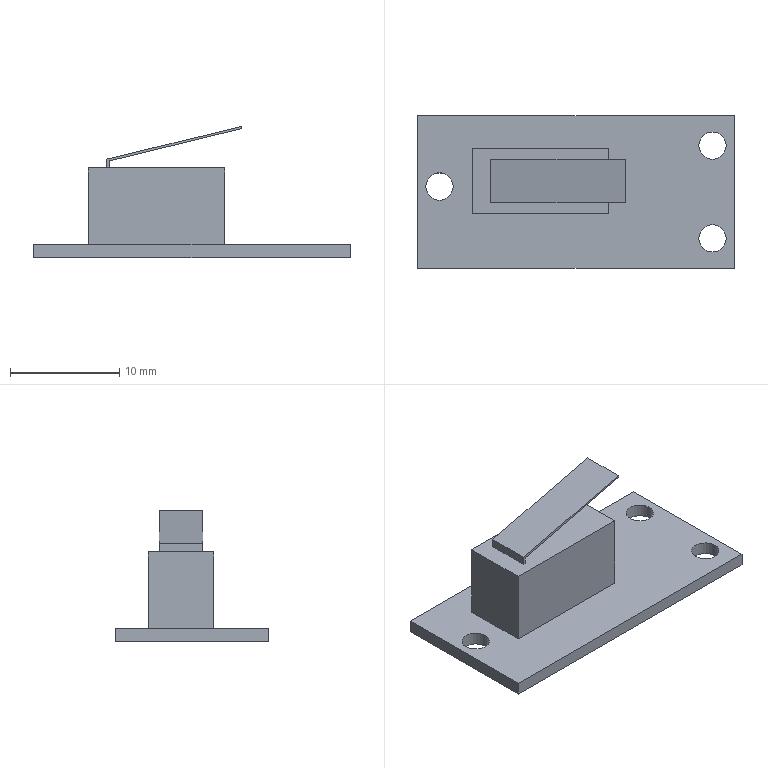Part | STEP file | Q7C1213W | 1 solid | 21 faces | box 29 x 14 x 12 mm | volume 1005 mm3 | plane 18 | cylinder 3 | commonest cylinder face diameters 2.5 x3
STEP:
#1=CARTESIAN_POINT('',(0.,0.,0.));
#2=DIRECTION('',(0.,0.,1.));
#3=DIRECTION('',(1.,0.,0.));
#4=AXIS2_PLACEMENT_3D('',#1,#2,#3);
#5=CARTESIAN_POINT('',(-11.25,0.5,1.2));
#6=VERTEX_POINT('',#5);
#7=CARTESIAN_POINT('',(-12.5,0.5,1.2));
#8=DIRECTION('',(0.,0.,1.));
#9=DIRECTION('',(1.,0.,0.));
#10=AXIS2_PLACEMENT_3D('',#7,#8,#9);
#11=CIRCLE('',#10,1.25);
#12=CARTESIAN_POINT('',(-14.5,-7.,1.2));
#13=DIRECTION('',(0.,0.,1.));
#14=DIRECTION('',(1.,0.,0.));
#15=AXIS2_PLACEMENT_3D('',#12,#13,#14);
#16=PLANE('',#15);
#17=CARTESIAN_POINT('',(2.,7.5));
#18=DIRECTION('',(1.,0.));
#19=AXIS2_PLACEMENT_2D('',#17,#18);
#20=CIRCLE('',#19,1.25);
#21=(GEOMETRIC_REPRESENTATION_CONTEXT(2)PARAMETRIC_REPRESENTATION_CONTEXT()REPRESENTATION_CONTEXT('',''));
#22=DEFINITIONAL_REPRESENTATION('',(#20),#21);
#23=PCURVE('',#16,#22);
#24=CARTESIAN_POINT('',(-12.5,0.5,1.2));
#25=DIRECTION('',(0.,0.,-1.));
#26=DIRECTION('',(-1.,0.,0.));
#27=AXIS2_PLACEMENT_3D('',#24,#25,#26);
#28=CYLINDRICAL_SURFACE('',#27,1.25);
#29=CARTESIAN_POINT('',(9.425,0.));
#30=DIRECTION('',(-1.,0.));
#31=VECTOR('',#30,1.);
#32=LINE('',#29,#31);
#33=(GEOMETRIC_REPRESENTATION_CONTEXT(2)PARAMETRIC_REPRESENTATION_CONTEXT()REPRESENTATION_CONTEXT('',''));
#34=DEFINITIONAL_REPRESENTATION('',(#32),#33);
#35=PCURVE('',#28,#34);
#36=SURFACE_CURVE('',#11,(#23,#35),.PCURVE_S1.);
#37=EDGE_CURVE('',#6,#6,#36,.T.);
#38=ORIENTED_EDGE('',*,*,#37,.F.);
#39=EDGE_LOOP('',(#38));
#40=FACE_BOUND('',#39,.T.);
#41=CARTESIAN_POINT('',(13.75,4.25,1.2));
#42=VERTEX_POINT('',#41);
#43=CARTESIAN_POINT('',(12.5,4.25,1.2));
#44=DIRECTION('',(0.,0.,1.));
#45=DIRECTION('',(1.,0.,0.));
#46=AXIS2_PLACEMENT_3D('',#43,#44,#45);
#47=CIRCLE('',#46,1.25);
#48=CARTESIAN_POINT('',(27.,11.25));
#49=DIRECTION('',(1.,0.));
#50=AXIS2_PLACEMENT_2D('',#48,#49);
#51=CIRCLE('',#50,1.25);
#52=(GEOMETRIC_REPRESENTATION_CONTEXT(2)PARAMETRIC_REPRESENTATION_CONTEXT()REPRESENTATION_CONTEXT('',''));
#53=DEFINITIONAL_REPRESENTATION('',(#51),#52);
#54=PCURVE('',#16,#53);
#55=CARTESIAN_POINT('',(12.5,4.25,1.2));
#56=DIRECTION('',(0.,0.,-1.));
#57=DIRECTION('',(-1.,0.,0.));
#58=AXIS2_PLACEMENT_3D('',#55,#56,#57);
#59=CYLINDRICAL_SURFACE('',#58,1.25);
#60=CARTESIAN_POINT('',(9.425,0.));
#61=DIRECTION('',(-1.,0.));
#62=VECTOR('',#61,1.);
#63=LINE('',#60,#62);
#64=(GEOMETRIC_REPRESENTATION_CONTEXT(2)PARAMETRIC_REPRESENTATION_CONTEXT()REPRESENTATION_CONTEXT('',''));
#65=DEFINITIONAL_REPRESENTATION('',(#63),#64);
#66=PCURVE('',#59,#65);
#67=SURFACE_CURVE('',#47,(#54,#66),.PCURVE_S1.);
#68=EDGE_CURVE('',#42,#42,#67,.T.);
#69=ORIENTED_EDGE('',*,*,#68,.F.);
#70=EDGE_LOOP('',(#69));
#71=FACE_BOUND('',#70,.T.);
#72=CARTESIAN_POINT('',(-14.5,7.,1.2));
#73=VERTEX_POINT('',#72);
#74=CARTESIAN_POINT('',(-14.5,-7.,1.2));
#75=VERTEX_POINT('',#74);
#76=CARTESIAN_POINT('',(-14.5,7.,1.2));
#77=DIRECTION('',(0.,-1.,0.));
#78=VECTOR('',#77,1.);
#79=LINE('',#76,#78);
#80=CARTESIAN_POINT('',(0.,14.));
#81=DIRECTION('',(0.,-1.));
#82=VECTOR('',#81,1.);
#83=LINE('',#80,#82);
#84=(GEOMETRIC_REPRESENTATION_CONTEXT(2)PARAMETRIC_REPRESENTATION_CONTEXT()REPRESENTATION_CONTEXT('',''));
#85=DEFINITIONAL_REPRESENTATION('',(#83),#84);
#86=PCURVE('',#16,#85);
#87=CARTESIAN_POINT('',(-14.5,7.,1.2));
#88=DIRECTION('',(1.,0.,0.));
#89=DIRECTION('',(0.,1.,0.));
#90=AXIS2_PLACEMENT_3D('',#87,#88,#89);
#91=PLANE('',#90);
#92=CARTESIAN_POINT('',(0.,0.));
#93=DIRECTION('',(-1.,0.));
#94=VECTOR('',#93,1.);
#95=LINE('',#92,#94);
#96=(GEOMETRIC_REPRESENTATION_CONTEXT(2)PARAMETRIC_REPRESENTATION_CONTEXT()REPRESENTATION_CONTEXT('',''));
#97=DEFINITIONAL_REPRESENTATION('',(#95),#96);
#98=PCURVE('',#91,#97);
#99=SURFACE_CURVE('',#79,(#86,#98),.PCURVE_S1.);
#100=EDGE_CURVE('',#73,#75,#99,.T.);
#101=ORIENTED_EDGE('',*,*,#100,.T.);
#102=CARTESIAN_POINT('',(14.5,-7.,1.2));
#103=VERTEX_POINT('',#102);
#104=CARTESIAN_POINT('',(-14.5,-7.,1.2));
#105=DIRECTION('',(1.,0.,0.));
#106=VECTOR('',#105,1.);
#107=LINE('',#104,#106);
#108=CARTESIAN_POINT('',(0.,0.));
#109=DIRECTION('',(1.,0.));
#110=VECTOR('',#109,1.);
#111=LINE('',#108,#110);
#112=(GEOMETRIC_REPRESENTATION_CONTEXT(2)PARAMETRIC_REPRESENTATION_CONTEXT()REPRESENTATION_CONTEXT('',''));
#113=DEFINITIONAL_REPRESENTATION('',(#111),#112);
#114=PCURVE('',#16,#113);
#115=CARTESIAN_POINT('',(-14.5,-7.,1.2));
#116=DIRECTION('',(0.,1.,0.));
#117=DIRECTION('',(0.,0.,1.));
#118=AXIS2_PLACEMENT_3D('',#115,#116,#117);
#119=PLANE('',#118);
#120=CARTESIAN_POINT('',(0.,0.));
#121=DIRECTION('',(0.,1.));
#122=VECTOR('',#121,1.);
#123=LINE('',#120,#122);
#124=(GEOMETRIC_REPRESENTATION_CONTEXT(2)PARAMETRIC_REPRESENTATION_CONTEXT()REPRESENTATION_CONTEXT('',''));
#125=DEFINITIONAL_REPRESENTATION('',(#123),#124);
#126=PCURVE('',#119,#125);
#127=SURFACE_CURVE('',#107,(#114,#126),.PCURVE_S1.);
#128=EDGE_CURVE('',#75,#103,#127,.T.);
#129=ORIENTED_EDGE('',*,*,#128,.T.);
#130=CARTESIAN_POINT('',(14.5,7.,1.2));
#131=VERTEX_POINT('',#130);
#132=CARTESIAN_POINT('',(14.5,7.,1.2));
#133=DIRECTION('',(0.,1.,0.));
#134=VECTOR('',#133,1.);
#135=LINE('',#132,#134);
#136=CARTESIAN_POINT('',(29.,14.));
#137=DIRECTION('',(0.,1.));
#138=VECTOR('',#137,1.);
#139=LINE('',#136,#138);
#140=(GEOMETRIC_REPRESENTATION_CONTEXT(2)PARAMETRIC_REPRESENTATION_CONTEXT()REPRESENTATION_CONTEXT('',''));
#141=DEFINITIONAL_REPRESENTATION('',(#139),#140);
#142=PCURVE('',#16,#141);
#143=CARTESIAN_POINT('',(14.5,7.,1.2));
#144=DIRECTION('',(-1.,0.,0.));
#145=DIRECTION('',(0.,-1.,0.));
#146=AXIS2_PLACEMENT_3D('',#143,#144,#145);
#147=PLANE('',#146);
#148=CARTESIAN_POINT('',(0.,0.));
#149=DIRECTION('',(-1.,0.));
#150=VECTOR('',#149,1.);
#151=LINE('',#148,#150);
#152=(GEOMETRIC_REPRESENTATION_CONTEXT(2)PARAMETRIC_REPRESENTATION_CONTEXT()REPRESENTATION_CONTEXT('',''));
#153=DEFINITIONAL_REPRESENTATION('',(#151),#152);
#154=PCURVE('',#147,#153);
#155=SURFACE_CURVE('',#135,(#142,#154),.PCURVE_S1.);
#156=EDGE_CURVE('',#103,#131,#155,.T.);
#157=ORIENTED_EDGE('',*,*,#156,.T.);
#158=CARTESIAN_POINT('',(-14.5,7.,1.2));
#159=DIRECTION('',(-1.,0.,0.));
#160=VECTOR('',#159,1.);
#161=LINE('',#158,#160);
#162=CARTESIAN_POINT('',(0.,14.));
#163=DIRECTION('',(-1.,0.));
#164=VECTOR('',#163,1.);
#165=LINE('',#162,#164);
#166=(GEOMETRIC_REPRESENTATION_CONTEXT(2)PARAMETRIC_REPRESENTATION_CONTEXT()REPRESENTATION_CONTEXT('',''));
#167=DEFINITIONAL_REPRESENTATION('',(#165),#166);
#168=PCURVE('',#16,#167);
#169=CARTESIAN_POINT('',(-14.5,7.,1.2));
#170=DIRECTION('',(0.,-1.,0.));
#171=DIRECTION('',(0.,0.,-1.));
#172=AXIS2_PLACEMENT_3D('',#169,#170,#171);
#173=PLANE('',#172);
#174=CARTESIAN_POINT('',(0.,0.));
#175=DIRECTION('',(0.,-1.));
#176=VECTOR('',#175,1.);
#177=LINE('',#174,#176);
#178=(GEOMETRIC_REPRESENTATION_CONTEXT(2)PARAMETRIC_REPRESENTATION_CONTEXT()REPRESENTATION_CONTEXT('',''));
#179=DEFINITIONAL_REPRESENTATION('',(#177),#178);
#180=PCURVE('',#173,#179);
#181=SURFACE_CURVE('',#161,(#168,#180),.PCURVE_S1.);
#182=EDGE_CURVE('',#131,#73,#181,.T.);
#183=ORIENTED_EDGE('',*,*,#182,.T.);
#184=EDGE_LOOP('',(#101,#129,#157,#183));
#185=FACE_BOUND('',#184,.T.);
#186=CARTESIAN_POINT('',(13.75,-4.25,1.2));
#187=VERTEX_POINT('',#186);
#188=CARTESIAN_POINT('',(12.5,-4.25,1.2));
#189=DIRECTION('',(0.,0.,1.));
#190=DIRECTION('',(1.,0.,0.));
#191=AXIS2_PLACEMENT_3D('',#188,#189,#190);
#192=CIRCLE('',#191,1.25);
#193=CARTESIAN_POINT('',(27.,2.75));
#194=DIRECTION('',(1.,0.));
#195=AXIS2_PLACEMENT_2D('',#193,#194);
#196=CIRCLE('',#195,1.25);
#197=(GEOMETRIC_REPRESENTATION_CONTEXT(2)PARAMETRIC_REPRESENTATION_CONTEXT()REPRESENTATION_CONTEXT('',''));
#198=DEFINITIONAL_REPRESENTATION('',(#196),#197);
#199=PCURVE('',#16,#198);
#200=CARTESIAN_POINT('',(12.5,-4.25,1.2));
#201=DIRECTION('',(0.,0.,-1.));
#202=DIRECTION('',(-1.,0.,0.));
#203=AXIS2_PLACEMENT_3D('',#200,#201,#202);
#204=CYLINDRICAL_SURFACE('',#203,1.25);
#205=CARTESIAN_POINT('',(9.425,0.));
#206=DIRECTION('',(-1.,0.));
#207=VECTOR('',#206,1.);
#208=LINE('',#205,#207);
#209=(GEOMETRIC_REPRESENTATION_CONTEXT(2)PARAMETRIC_REPRESENTATION_CONTEXT()REPRESENTATION_CONTEXT('',''));
#210=DEFINITIONAL_REPRESENTATION('',(#208),#209);
#211=PCURVE('',#204,#210);
#212=SURFACE_CURVE('',#192,(#199,#211),.PCURVE_S1.);
#213=EDGE_CURVE('',#187,#187,#212,.T.);
#214=ORIENTED_EDGE('',*,*,#213,.F.);
#215=EDGE_LOOP('',(#214));
#216=FACE_BOUND('',#215,.T.);
#217=CARTESIAN_POINT('',(-9.5,-2.,1.2));
#218=VERTEX_POINT('',#217);
#219=CARTESIAN_POINT('',(3.,-2.,1.2));
#220=VERTEX_POINT('',#219);
#221=CARTESIAN_POINT('',(-9.5,-2.,1.2));
#222=DIRECTION('',(1.,0.,0.));
#223=VECTOR('',#222,1.);
#224=LINE('',#221,#223);
#225=CARTESIAN_POINT('',(5.,5.));
#226=DIRECTION('',(1.,0.));
#227=VECTOR('',#226,1.);
#228=LINE('',#225,#227);
#229=(GEOMETRIC_REPRESENTATION_CONTEXT(2)PARAMETRIC_REPRESENTATION_CONTEXT()REPRESENTATION_CONTEXT('',''));
#230=DEFINITIONAL_REPRESENTATION('',(#228),#229);
#231=PCURVE('',#16,#230);
#232=CARTESIAN_POINT('',(-9.5,-2.,8.2));
#233=DIRECTION('',(0.,1.,0.));
#234=DIRECTION('',(0.,0.,1.));
#235=AXIS2_PLACEMENT_3D('',#232,#233,#234);
#236=PLANE('',#235);
#237=CARTESIAN_POINT('',(-7.,0.));
#238=DIRECTION('',(0.,1.));
#239=VECTOR('',#238,1.);
#240=LINE('',#237,#239);
#241=(GEOMETRIC_REPRESENTATION_CONTEXT(2)PARAMETRIC_REPRESENTATION_CONTEXT()REPRESENTATION_CONTEXT('',''));
#242=DEFINITIONAL_REPRESENTATION('',(#240),#241);
#243=PCURVE('',#236,#242);
#244=SURFACE_CURVE('',#224,(#231,#243),.PCURVE_S1.);
#245=EDGE_CURVE('',#218,#220,#244,.T.);
#246=ORIENTED_EDGE('',*,*,#245,.F.);
#247=CARTESIAN_POINT('',(-9.5,4.,1.2));
#248=VERTEX_POINT('',#247);
#249=CARTESIAN_POINT('',(-9.5,4.,1.2));
#250=DIRECTION('',(0.,-1.,0.));
#251=VECTOR('',#250,1.);
#252=LINE('',#249,#251);
#253=CARTESIAN_POINT('',(5.,11.));
#254=DIRECTION('',(0.,-1.));
#255=VECTOR('',#254,1.);
#256=LINE('',#253,#255);
#257=(GEOMETRIC_REPRESENTATION_CONTEXT(2)PARAMETRIC_REPRESENTATION_CONTEXT()REPRESENTATION_CONTEXT('',''));
#258=DEFINITIONAL_REPRESENTATION('',(#256),#257);
#259=PCURVE('',#16,#258);
#260=CARTESIAN_POINT('',(-9.5,4.,8.2));
#261=DIRECTION('',(1.,0.,0.));
#262=DIRECTION('',(0.,0.,-1.));
#263=AXIS2_PLACEMENT_3D('',#260,#261,#262);
#264=PLANE('',#263);
#265=CARTESIAN_POINT('',(7.,0.));
#266=DIRECTION('',(0.,-1.));
#267=VECTOR('',#266,1.);
#268=LINE('',#265,#267);
#269=(GEOMETRIC_REPRESENTATION_CONTEXT(2)PARAMETRIC_REPRESENTATION_CONTEXT()REPRESENTATION_CONTEXT('',''));
#270=DEFINITIONAL_REPRESENTATION('',(#268),#269);
#271=PCURVE('',#264,#270);
#272=SURFACE_CURVE('',#252,(#259,#271),.PCURVE_S1.);
#273=EDGE_CURVE('',#248,#218,#272,.T.);
#274=ORIENTED_EDGE('',*,*,#273,.F.);
#275=CARTESIAN_POINT('',(3.,4.,1.2));
#276=VERTEX_POINT('',#275);
#277=CARTESIAN_POINT('',(-9.5,4.,1.2));
#278=DIRECTION('',(-1.,0.,0.));
#279=VECTOR('',#278,1.);
#280=LINE('',#277,#279);
#281=CARTESIAN_POINT('',(5.,11.));
#282=DIRECTION('',(-1.,0.));
#283=VECTOR('',#282,1.);
#284=LINE('',#281,#283);
#285=(GEOMETRIC_REPRESENTATION_CONTEXT(2)PARAMETRIC_REPRESENTATION_CONTEXT()REPRESENTATION_CONTEXT('',''));
#286=DEFINITIONAL_REPRESENTATION('',(#284),#285);
#287=PCURVE('',#16,#286);
#288=CARTESIAN_POINT('',(-9.5,4.,8.2));
#289=DIRECTION('',(0.,-1.,0.));
#290=DIRECTION('',(0.,0.,-1.));
#291=AXIS2_PLACEMENT_3D('',#288,#289,#290);
#292=PLANE('',#291);
#293=CARTESIAN_POINT('',(7.,0.));
#294=DIRECTION('',(0.,-1.));
#295=VECTOR('',#294,1.);
#296=LINE('',#293,#295);
#297=(GEOMETRIC_REPRESENTATION_CONTEXT(2)PARAMETRIC_REPRESENTATION_CONTEXT()REPRESENTATION_CONTEXT('',''));
#298=DEFINITIONAL_REPRESENTATION('',(#296),#297);
#299=PCURVE('',#292,#298);
#300=SURFACE_CURVE('',#280,(#287,#299),.PCURVE_S1.);
#301=EDGE_CURVE('',#276,#248,#300,.T.);
#302=ORIENTED_EDGE('',*,*,#301,.F.);
#303=CARTESIAN_POINT('',(3.,4.,1.2));
#304=DIRECTION('',(0.,1.,0.));
#305=VECTOR('',#304,1.);
#306=LINE('',#303,#305);
#307=CARTESIAN_POINT('',(17.5,11.));
#308=DIRECTION('',(0.,1.));
#309=VECTOR('',#308,1.);
#310=LINE('',#307,#309);
#311=(GEOMETRIC_REPRESENTATION_CONTEXT(2)PARAMETRIC_REPRESENTATION_CONTEXT()REPRESENTATION_CONTEXT('',''));
#312=DEFINITIONAL_REPRESENTATION('',(#310),#311);
#313=PCURVE('',#16,#312);
#314=CARTESIAN_POINT('',(3.,4.,8.2));
#315=DIRECTION('',(-1.,0.,0.));
#316=DIRECTION('',(0.,0.,1.));
#317=AXIS2_PLACEMENT_3D('',#314,#315,#316);
#318=PLANE('',#317);
#319=CARTESIAN_POINT('',(-7.,0.));
#320=DIRECTION('',(0.,1.));
#321=VECTOR('',#320,1.);
#322=LINE('',#319,#321);
#323=(GEOMETRIC_REPRESENTATION_CONTEXT(2)PARAMETRIC_REPRESENTATION_CONTEXT()REPRESENTATION_CONTEXT('',''));
#324=DEFINITIONAL_REPRESENTATION('',(#322),#323);
#325=PCURVE('',#318,#324);
#326=SURFACE_CURVE('',#306,(#313,#325),.PCURVE_S1.);
#327=EDGE_CURVE('',#220,#276,#326,.T.);
#328=ORIENTED_EDGE('',*,*,#327,.F.);
#329=EDGE_LOOP('',(#246,#274,#302,#328));
#330=FACE_BOUND('',#329,.T.);
#331=ADVANCED_FACE('',(#40,#71,#185,#216,#330),#16,.T.);
#332=CARTESIAN_POINT('',(13.75,-4.25,0.));
#333=VERTEX_POINT('',#332);
#334=CARTESIAN_POINT('',(12.5,-4.25,0.));
#335=DIRECTION('',(0.,0.,1.));
#336=DIRECTION('',(1.,0.,0.));
#337=AXIS2_PLACEMENT_3D('',#334,#335,#336);
#338=CIRCLE('',#337,1.25);
#339=CARTESIAN_POINT('',(-14.5,-7.,0.));
#340=DIRECTION('',(0.,0.,1.));
#341=DIRECTION('',(1.,0.,0.));
#342=AXIS2_PLACEMENT_3D('',#339,#340,#341);
#343=PLANE('',#342);
#344=CARTESIAN_POINT('',(27.,2.75));
#345=DIRECTION('',(1.,0.));
#346=AXIS2_PLACEMENT_2D('',#344,#345);
#347=CIRCLE('',#346,1.25);
#348=(GEOMETRIC_REPRESENTATION_CONTEXT(2)PARAMETRIC_REPRESENTATION_CONTEXT()REPRESENTATION_CONTEXT('',''));
#349=DEFINITIONAL_REPRESENTATION('',(#347),#348);
#350=PCURVE('',#343,#349);
#351=CARTESIAN_POINT('',(9.425,1.2));
#352=DIRECTION('',(-1.,0.));
#353=VECTOR('',#352,1.);
#354=LINE('',#351,#353);
#355=(GEOMETRIC_REPRESENTATION_CONTEXT(2)PARAMETRIC_REPRESENTATION_CONTEXT()REPRESENTATION_CONTEXT('',''));
#356=DEFINITIONAL_REPRESENTATION('',(#354),#355);
#357=PCURVE('',#204,#356);
#358=SURFACE_CURVE('',#338,(#350,#357),.PCURVE_S1.);
#359=EDGE_CURVE('',#333,#333,#358,.T.);
#360=ORIENTED_EDGE('',*,*,#359,.T.);
#361=EDGE_LOOP('',(#360));
#362=FACE_BOUND('',#361,.T.);
#363=CARTESIAN_POINT('',(-14.5,7.,0.));
#364=VERTEX_POINT('',#363);
#365=CARTESIAN_POINT('',(-14.5,-7.,0.));
#366=VERTEX_POINT('',#365);
#367=CARTESIAN_POINT('',(-14.5,7.,0.));
#368=DIRECTION('',(0.,-1.,0.));
#369=VECTOR('',#368,1.);
#370=LINE('',#367,#369);
#371=CARTESIAN_POINT('',(0.,14.));
#372=DIRECTION('',(0.,-1.));
#373=VECTOR('',#372,1.);
#374=LINE('',#371,#373);
#375=(GEOMETRIC_REPRESENTATION_CONTEXT(2)PARAMETRIC_REPRESENTATION_CONTEXT()REPRESENTATION_CONTEXT('',''));
#376=DEFINITIONAL_REPRESENTATION('',(#374),#375);
#377=PCURVE('',#343,#376);
#378=CARTESIAN_POINT('',(0.,-1.2));
#379=DIRECTION('',(-1.,0.));
#380=VECTOR('',#379,1.);
#381=LINE('',#378,#380);
#382=(GEOMETRIC_REPRESENTATION_CONTEXT(2)PARAMETRIC_REPRESENTATION_CONTEXT()REPRESENTATION_CONTEXT('',''));
#383=DEFINITIONAL_REPRESENTATION('',(#381),#382);
#384=PCURVE('',#91,#383);
#385=SURFACE_CURVE('',#370,(#377,#384),.PCURVE_S1.);
#386=EDGE_CURVE('',#364,#366,#385,.T.);
#387=ORIENTED_EDGE('',*,*,#386,.F.);
#388=CARTESIAN_POINT('',(14.5,7.,0.));
#389=VERTEX_POINT('',#388);
#390=CARTESIAN_POINT('',(-14.5,7.,0.));
#391=DIRECTION('',(-1.,0.,0.));
#392=VECTOR('',#391,1.);
#393=LINE('',#390,#392);
#394=CARTESIAN_POINT('',(0.,14.));
#395=DIRECTION('',(-1.,0.));
#396=VECTOR('',#395,1.);
#397=LINE('',#394,#396);
#398=(GEOMETRIC_REPRESENTATION_CONTEXT(2)PARAMETRIC_REPRESENTATION_CONTEXT()REPRESENTATION_CONTEXT('',''));
#399=DEFINITIONAL_REPRESENTATION('',(#397),#398);
#400=PCURVE('',#343,#399);
#401=CARTESIAN_POINT('',(1.2,0.));
#402=DIRECTION('',(0.,-1.));
#403=VECTOR('',#402,1.);
#404=LINE('',#401,#403);
#405=(GEOMETRIC_REPRESENTATION_CONTEXT(2)PARAMETRIC_REPRESENTATION_CONTEXT()REPRESENTATION_CONTEXT('',''));
#406=DEFINITIONAL_REPRESENTATION('',(#404),#405);
#407=PCURVE('',#173,#406);
#408=SURFACE_CURVE('',#393,(#400,#407),.PCURVE_S1.);
#409=EDGE_CURVE('',#389,#364,#408,.T.);
#410=ORIENTED_EDGE('',*,*,#409,.F.);
#411=CARTESIAN_POINT('',(14.5,-7.,0.));
#412=VERTEX_POINT('',#411);
#413=CARTESIAN_POINT('',(14.5,7.,0.));
#414=DIRECTION('',(0.,1.,0.));
#415=VECTOR('',#414,1.);
#416=LINE('',#413,#415);
#417=CARTESIAN_POINT('',(29.,14.));
#418=DIRECTION('',(0.,1.));
#419=VECTOR('',#418,1.);
#420=LINE('',#417,#419);
#421=(GEOMETRIC_REPRESENTATION_CONTEXT(2)PARAMETRIC_REPRESENTATION_CONTEXT()REPRESENTATION_CONTEXT('',''));
#422=DEFINITIONAL_REPRESENTATION('',(#420),#421);
#423=PCURVE('',#343,#422);
#424=CARTESIAN_POINT('',(0.,-1.2));
#425=DIRECTION('',(-1.,0.));
#426=VECTOR('',#425,1.);
#427=LINE('',#424,#426);
#428=(GEOMETRIC_REPRESENTATION_CONTEXT(2)PARAMETRIC_REPRESENTATION_CONTEXT()REPRESENTATION_CONTEXT('',''));
#429=DEFINITIONAL_REPRESENTATION('',(#427),#428);
#430=PCURVE('',#147,#429);
#431=SURFACE_CURVE('',#416,(#423,#430),.PCURVE_S1.);
#432=EDGE_CURVE('',#412,#389,#431,.T.);
#433=ORIENTED_EDGE('',*,*,#432,.F.);
#434=CARTESIAN_POINT('',(-14.5,-7.,0.));
#435=DIRECTION('',(1.,0.,0.));
#436=VECTOR('',#435,1.);
#437=LINE('',#434,#436);
#438=CARTESIAN_POINT('',(0.,0.));
#439=DIRECTION('',(1.,0.));
#440=VECTOR('',#439,1.);
#441=LINE('',#438,#440);
#442=(GEOMETRIC_REPRESENTATION_CONTEXT(2)PARAMETRIC_REPRESENTATION_CONTEXT()REPRESENTATION_CONTEXT('',''));
#443=DEFINITIONAL_REPRESENTATION('',(#441),#442);
#444=PCURVE('',#343,#443);
#445=CARTESIAN_POINT('',(-1.2,0.));
#446=DIRECTION('',(0.,1.));
#447=VECTOR('',#446,1.);
#448=LINE('',#445,#447);
#449=(GEOMETRIC_REPRESENTATION_CONTEXT(2)PARAMETRIC_REPRESENTATION_CONTEXT()REPRESENTATION_CONTEXT('',''));
#450=DEFINITIONAL_REPRESENTATION('',(#448),#449);
#451=PCURVE('',#119,#450);
#452=SURFACE_CURVE('',#437,(#444,#451),.PCURVE_S1.);
#453=EDGE_CURVE('',#366,#412,#452,.T.);
#454=ORIENTED_EDGE('',*,*,#453,.F.);
#455=EDGE_LOOP('',(#387,#410,#433,#454));
#456=FACE_BOUND('',#455,.T.);
#457=CARTESIAN_POINT('',(13.75,4.25,0.));
#458=VERTEX_POINT('',#457);
#459=CARTESIAN_POINT('',(12.5,4.25,0.));
#460=DIRECTION('',(0.,0.,1.));
#461=DIRECTION('',(1.,0.,0.));
#462=AXIS2_PLACEMENT_3D('',#459,#460,#461);
#463=CIRCLE('',#462,1.25);
#464=CARTESIAN_POINT('',(27.,11.25));
#465=DIRECTION('',(1.,0.));
#466=AXIS2_PLACEMENT_2D('',#464,#465);
#467=CIRCLE('',#466,1.25);
#468=(GEOMETRIC_REPRESENTATION_CONTEXT(2)PARAMETRIC_REPRESENTATION_CONTEXT()REPRESENTATION_CONTEXT('',''));
#469=DEFINITIONAL_REPRESENTATION('',(#467),#468);
#470=PCURVE('',#343,#469);
#471=CARTESIAN_POINT('',(9.425,1.2));
#472=DIRECTION('',(-1.,0.));
#473=VECTOR('',#472,1.);
#474=LINE('',#471,#473);
#475=(GEOMETRIC_REPRESENTATION_CONTEXT(2)PARAMETRIC_REPRESENTATION_CONTEXT()REPRESENTATION_CONTEXT('',''));
#476=DEFINITIONAL_REPRESENTATION('',(#474),#475);
#477=PCURVE('',#59,#476);
#478=SURFACE_CURVE('',#463,(#470,#477),.PCURVE_S1.);
#479=EDGE_CURVE('',#458,#458,#478,.T.);
#480=ORIENTED_EDGE('',*,*,#479,.T.);
#481=EDGE_LOOP('',(#480));
#482=FACE_BOUND('',#481,.T.);
#483=CARTESIAN_POINT('',(-11.25,0.5,0.));
#484=VERTEX_POINT('',#483);
#485=CARTESIAN_POINT('',(-12.5,0.5,0.));
#486=DIRECTION('',(0.,0.,1.));
#487=DIRECTION('',(1.,0.,0.));
#488=AXIS2_PLACEMENT_3D('',#485,#486,#487);
#489=CIRCLE('',#488,1.25);
#490=CARTESIAN_POINT('',(2.,7.5));
#491=DIRECTION('',(1.,0.));
#492=AXIS2_PLACEMENT_2D('',#490,#491);
#493=CIRCLE('',#492,1.25);
#494=(GEOMETRIC_REPRESENTATION_CONTEXT(2)PARAMETRIC_REPRESENTATION_CONTEXT()REPRESENTATION_CONTEXT('',''));
#495=DEFINITIONAL_REPRESENTATION('',(#493),#494);
#496=PCURVE('',#343,#495);
#497=CARTESIAN_POINT('',(9.425,1.2));
#498=DIRECTION('',(-1.,0.));
#499=VECTOR('',#498,1.);
#500=LINE('',#497,#499);
#501=(GEOMETRIC_REPRESENTATION_CONTEXT(2)PARAMETRIC_REPRESENTATION_CONTEXT()REPRESENTATION_CONTEXT('',''));
#502=DEFINITIONAL_REPRESENTATION('',(#500),#501);
#503=PCURVE('',#28,#502);
#504=SURFACE_CURVE('',#489,(#496,#503),.PCURVE_S1.);
#505=EDGE_CURVE('',#484,#484,#504,.T.);
#506=ORIENTED_EDGE('',*,*,#505,.T.);
#507=EDGE_LOOP('',(#506));
#508=FACE_BOUND('',#507,.T.);
#509=ADVANCED_FACE('',(#362,#456,#482,#508),#343,.F.);
#510=ORIENTED_EDGE('',*,*,#386,.T.);
#511=CARTESIAN_POINT('',(-14.5,-7.,1.2));
#512=DIRECTION('',(0.,0.,-1.));
#513=VECTOR('',#512,1.);
#514=LINE('',#511,#513);
#515=CARTESIAN_POINT('',(-14.,0.));
#516=DIRECTION('',(0.,-1.));
#517=VECTOR('',#516,1.);
#518=LINE('',#515,#517);
#519=(GEOMETRIC_REPRESENTATION_CONTEXT(2)PARAMETRIC_REPRESENTATION_CONTEXT()REPRESENTATION_CONTEXT('',''));
#520=DEFINITIONAL_REPRESENTATION('',(#518),#519);
#521=PCURVE('',#91,#520);
#522=CARTESIAN_POINT('',(0.,0.));
#523=DIRECTION('',(-1.,0.));
#524=VECTOR('',#523,1.);
#525=LINE('',#522,#524);
#526=(GEOMETRIC_REPRESENTATION_CONTEXT(2)PARAMETRIC_REPRESENTATION_CONTEXT()REPRESENTATION_CONTEXT('',''));
#527=DEFINITIONAL_REPRESENTATION('',(#525),#526);
#528=PCURVE('',#119,#527);
#529=SURFACE_CURVE('',#514,(#521,#528),.PCURVE_S1.);
#530=EDGE_CURVE('',#75,#366,#529,.T.);
#531=ORIENTED_EDGE('',*,*,#530,.F.);
#532=ORIENTED_EDGE('',*,*,#100,.F.);
#533=CARTESIAN_POINT('',(-14.5,7.,1.2));
#534=DIRECTION('',(0.,0.,-1.));
#535=VECTOR('',#534,1.);
#536=LINE('',#533,#535);
#537=CARTESIAN_POINT('',(0.,0.));
#538=DIRECTION('',(0.,-1.));
#539=VECTOR('',#538,1.);
#540=LINE('',#537,#539);
#541=(GEOMETRIC_REPRESENTATION_CONTEXT(2)PARAMETRIC_REPRESENTATION_CONTEXT()REPRESENTATION_CONTEXT('',''));
#542=DEFINITIONAL_REPRESENTATION('',(#540),#541);
#543=PCURVE('',#91,#542);
#544=CARTESIAN_POINT('',(0.,0.));
#545=DIRECTION('',(1.,0.));
#546=VECTOR('',#545,1.);
#547=LINE('',#544,#546);
#548=(GEOMETRIC_REPRESENTATION_CONTEXT(2)PARAMETRIC_REPRESENTATION_CONTEXT()REPRESENTATION_CONTEXT('',''));
#549=DEFINITIONAL_REPRESENTATION('',(#547),#548);
#550=PCURVE('',#173,#549);
#551=SURFACE_CURVE('',#536,(#543,#550),.PCURVE_S1.);
#552=EDGE_CURVE('',#73,#364,#551,.T.);
#553=ORIENTED_EDGE('',*,*,#552,.T.);
#554=EDGE_LOOP('',(#510,#531,#532,#553));
#555=FACE_BOUND('',#554,.T.);
#556=ADVANCED_FACE('',(#555),#91,.F.);
#557=ORIENTED_EDGE('',*,*,#453,.T.);
#558=CARTESIAN_POINT('',(14.5,-7.,1.2));
#559=DIRECTION('',(0.,0.,-1.));
#560=VECTOR('',#559,1.);
#561=LINE('',#558,#560);
#562=CARTESIAN_POINT('',(0.,29.));
#563=DIRECTION('',(-1.,0.));
#564=VECTOR('',#563,1.);
#565=LINE('',#562,#564);
#566=(GEOMETRIC_REPRESENTATION_CONTEXT(2)PARAMETRIC_REPRESENTATION_CONTEXT()REPRESENTATION_CONTEXT('',''));
#567=DEFINITIONAL_REPRESENTATION('',(#565),#566);
#568=PCURVE('',#119,#567);
#569=CARTESIAN_POINT('',(14.,0.));
#570=DIRECTION('',(0.,-1.));
#571=VECTOR('',#570,1.);
#572=LINE('',#569,#571);
#573=(GEOMETRIC_REPRESENTATION_CONTEXT(2)PARAMETRIC_REPRESENTATION_CONTEXT()REPRESENTATION_CONTEXT('',''));
#574=DEFINITIONAL_REPRESENTATION('',(#572),#573);
#575=PCURVE('',#147,#574);
#576=SURFACE_CURVE('',#561,(#568,#575),.PCURVE_S1.);
#577=EDGE_CURVE('',#103,#412,#576,.T.);
#578=ORIENTED_EDGE('',*,*,#577,.F.);
#579=ORIENTED_EDGE('',*,*,#128,.F.);
#580=ORIENTED_EDGE('',*,*,#530,.T.);
#581=EDGE_LOOP('',(#557,#578,#579,#580));
#582=FACE_BOUND('',#581,.T.);
#583=ADVANCED_FACE('',(#582),#119,.F.);
#584=ORIENTED_EDGE('',*,*,#432,.T.);
#585=CARTESIAN_POINT('',(14.5,7.,1.2));
#586=DIRECTION('',(0.,0.,-1.));
#587=VECTOR('',#586,1.);
#588=LINE('',#585,#587);
#589=CARTESIAN_POINT('',(0.,0.));
#590=DIRECTION('',(0.,-1.));
#591=VECTOR('',#590,1.);
#592=LINE('',#589,#591);
#593=(GEOMETRIC_REPRESENTATION_CONTEXT(2)PARAMETRIC_REPRESENTATION_CONTEXT()REPRESENTATION_CONTEXT('',''));
#594=DEFINITIONAL_REPRESENTATION('',(#592),#593);
#595=PCURVE('',#147,#594);
#596=CARTESIAN_POINT('',(0.,29.));
#597=DIRECTION('',(1.,0.));
#598=VECTOR('',#597,1.);
#599=LINE('',#596,#598);
#600=(GEOMETRIC_REPRESENTATION_CONTEXT(2)PARAMETRIC_REPRESENTATION_CONTEXT()REPRESENTATION_CONTEXT('',''));
#601=DEFINITIONAL_REPRESENTATION('',(#599),#600);
#602=PCURVE('',#173,#601);
#603=SURFACE_CURVE('',#588,(#595,#602),.PCURVE_S1.);
#604=EDGE_CURVE('',#131,#389,#603,.T.);
#605=ORIENTED_EDGE('',*,*,#604,.F.);
#606=ORIENTED_EDGE('',*,*,#156,.F.);
#607=ORIENTED_EDGE('',*,*,#577,.T.);
#608=EDGE_LOOP('',(#584,#605,#606,#607));
#609=FACE_BOUND('',#608,.T.);
#610=ADVANCED_FACE('',(#609),#147,.F.);
#611=ORIENTED_EDGE('',*,*,#409,.T.);
#612=ORIENTED_EDGE('',*,*,#552,.F.);
#613=ORIENTED_EDGE('',*,*,#182,.F.);
#614=ORIENTED_EDGE('',*,*,#604,.T.);
#615=EDGE_LOOP('',(#611,#612,#613,#614));
#616=FACE_BOUND('',#615,.T.);
#617=ADVANCED_FACE('',(#616),#173,.F.);
#618=ORIENTED_EDGE('',*,*,#68,.F.);
#619=CARTESIAN_POINT('',(13.75,4.25,1.2));
#620=CARTESIAN_POINT('',(13.75,4.25,0.));
#621=B_SPLINE_CURVE_WITH_KNOTS('',1,(#619,#620),.UNSPECIFIED.,.F.,.F.,(2,2),(0.,1.2),.PIECEWISE_BEZIER_KNOTS.);
#622=CARTESIAN_POINT('',(9.425,0.));
#623=DIRECTION('',(0.,1.));
#624=VECTOR('',#623,1.);
#625=LINE('',#622,#624);
#626=(GEOMETRIC_REPRESENTATION_CONTEXT(2)PARAMETRIC_REPRESENTATION_CONTEXT()REPRESENTATION_CONTEXT('',''));
#627=DEFINITIONAL_REPRESENTATION('',(#625),#626);
#628=PCURVE('',#59,#627);
#629=CARTESIAN_POINT('',(3.142,0.));
#630=DIRECTION('',(0.,1.));
#631=VECTOR('',#630,1.);
#632=LINE('',#629,#631);
#633=(GEOMETRIC_REPRESENTATION_CONTEXT(2)PARAMETRIC_REPRESENTATION_CONTEXT()REPRESENTATION_CONTEXT('',''));
#634=DEFINITIONAL_REPRESENTATION('',(#632),#633);
#635=PCURVE('',#59,#634);
#636=SEAM_CURVE('',#621,(#628,#635),.PCURVE_S1.);
#637=EDGE_CURVE('',#42,#458,#636,.T.);
#638=ORIENTED_EDGE('',*,*,#637,.T.);
#639=ORIENTED_EDGE('',*,*,#479,.T.);
#640=ORIENTED_EDGE('',*,*,#637,.F.);
#641=EDGE_LOOP('',(#618,#638,#639,#640));
#642=FACE_BOUND('',#641,.F.);
#643=ADVANCED_FACE('',(#642),#59,.F.);
#644=ORIENTED_EDGE('',*,*,#213,.F.);
#645=CARTESIAN_POINT('',(13.75,-4.25,1.2));
#646=CARTESIAN_POINT('',(13.75,-4.25,0.));
#647=B_SPLINE_CURVE_WITH_KNOTS('',1,(#645,#646),.UNSPECIFIED.,.F.,.F.,(2,2),(0.,1.2),.PIECEWISE_BEZIER_KNOTS.);
#648=CARTESIAN_POINT('',(9.425,0.));
#649=DIRECTION('',(0.,1.));
#650=VECTOR('',#649,1.);
#651=LINE('',#648,#650);
#652=(GEOMETRIC_REPRESENTATION_CONTEXT(2)PARAMETRIC_REPRESENTATION_CONTEXT()REPRESENTATION_CONTEXT('',''));
#653=DEFINITIONAL_REPRESENTATION('',(#651),#652);
#654=PCURVE('',#204,#653);
#655=CARTESIAN_POINT('',(3.142,0.));
#656=DIRECTION('',(0.,1.));
#657=VECTOR('',#656,1.);
#658=LINE('',#655,#657);
#659=(GEOMETRIC_REPRESENTATION_CONTEXT(2)PARAMETRIC_REPRESENTATION_CONTEXT()REPRESENTATION_CONTEXT('',''));
#660=DEFINITIONAL_REPRESENTATION('',(#658),#659);
#661=PCURVE('',#204,#660);
#662=SEAM_CURVE('',#647,(#654,#661),.PCURVE_S1.);
#663=EDGE_CURVE('',#187,#333,#662,.T.);
#664=ORIENTED_EDGE('',*,*,#663,.T.);
#665=ORIENTED_EDGE('',*,*,#359,.T.);
#666=ORIENTED_EDGE('',*,*,#663,.F.);
#667=EDGE_LOOP('',(#644,#664,#665,#666));
#668=FACE_BOUND('',#667,.F.);
#669=ADVANCED_FACE('',(#668),#204,.F.);
#670=ORIENTED_EDGE('',*,*,#37,.F.);
#671=CARTESIAN_POINT('',(-11.25,0.5,1.2));
#672=CARTESIAN_POINT('',(-11.25,0.5,0.));
#673=B_SPLINE_CURVE_WITH_KNOTS('',1,(#671,#672),.UNSPECIFIED.,.F.,.F.,(2,2),(0.,1.2),.PIECEWISE_BEZIER_KNOTS.);
#674=CARTESIAN_POINT('',(9.425,0.));
#675=DIRECTION('',(0.,1.));
#676=VECTOR('',#675,1.);
#677=LINE('',#674,#676);
#678=(GEOMETRIC_REPRESENTATION_CONTEXT(2)PARAMETRIC_REPRESENTATION_CONTEXT()REPRESENTATION_CONTEXT('',''));
#679=DEFINITIONAL_REPRESENTATION('',(#677),#678);
#680=PCURVE('',#28,#679);
#681=CARTESIAN_POINT('',(3.142,0.));
#682=DIRECTION('',(0.,1.));
#683=VECTOR('',#682,1.);
#684=LINE('',#681,#683);
#685=(GEOMETRIC_REPRESENTATION_CONTEXT(2)PARAMETRIC_REPRESENTATION_CONTEXT()REPRESENTATION_CONTEXT('',''));
#686=DEFINITIONAL_REPRESENTATION('',(#684),#685);
#687=PCURVE('',#28,#686);
#688=SEAM_CURVE('',#673,(#680,#687),.PCURVE_S1.);
#689=EDGE_CURVE('',#6,#484,#688,.T.);
#690=ORIENTED_EDGE('',*,*,#689,.T.);
#691=ORIENTED_EDGE('',*,*,#505,.T.);
#692=ORIENTED_EDGE('',*,*,#689,.F.);
#693=EDGE_LOOP('',(#670,#690,#691,#692));
#694=FACE_BOUND('',#693,.F.);
#695=ADVANCED_FACE('',(#694),#28,.F.);
#696=ORIENTED_EDGE('',*,*,#273,.T.);
#697=CARTESIAN_POINT('',(-9.5,-2.,8.2));
#698=VERTEX_POINT('',#697);
#699=CARTESIAN_POINT('',(-9.5,-2.,8.2));
#700=DIRECTION('',(0.,0.,-1.));
#701=VECTOR('',#700,1.);
#702=LINE('',#699,#701);
#703=CARTESIAN_POINT('',(0.,-6.));
#704=DIRECTION('',(1.,0.));
#705=VECTOR('',#704,1.);
#706=LINE('',#703,#705);
#707=(GEOMETRIC_REPRESENTATION_CONTEXT(2)PARAMETRIC_REPRESENTATION_CONTEXT()REPRESENTATION_CONTEXT('',''));
#708=DEFINITIONAL_REPRESENTATION('',(#706),#707);
#709=PCURVE('',#264,#708);
#710=CARTESIAN_POINT('',(0.,0.));
#711=DIRECTION('',(-1.,0.));
#712=VECTOR('',#711,1.);
#713=LINE('',#710,#712);
#714=(GEOMETRIC_REPRESENTATION_CONTEXT(2)PARAMETRIC_REPRESENTATION_CONTEXT()REPRESENTATION_CONTEXT('',''));
#715=DEFINITIONAL_REPRESENTATION('',(#713),#714);
#716=PCURVE('',#236,#715);
#717=SURFACE_CURVE('',#702,(#709,#716),.PCURVE_S1.);
#718=EDGE_CURVE('',#698,#218,#717,.T.);
#719=ORIENTED_EDGE('',*,*,#718,.F.);
#720=CARTESIAN_POINT('',(-9.5,4.,8.2));
#721=VERTEX_POINT('',#720);
#722=CARTESIAN_POINT('',(-9.5,4.,8.2));
#723=DIRECTION('',(0.,-1.,0.));
#724=VECTOR('',#723,1.);
#725=LINE('',#722,#724);
#726=CARTESIAN_POINT('',(0.,0.));
#727=DIRECTION('',(0.,-1.));
#728=VECTOR('',#727,1.);
#729=LINE('',#726,#728);
#730=(GEOMETRIC_REPRESENTATION_CONTEXT(2)PARAMETRIC_REPRESENTATION_CONTEXT()REPRESENTATION_CONTEXT('',''));
#731=DEFINITIONAL_REPRESENTATION('',(#729),#730);
#732=PCURVE('',#264,#731);
#733=CARTESIAN_POINT('',(-9.5,-2.,8.2));
#734=DIRECTION('',(0.,0.,1.));
#735=DIRECTION('',(1.,0.,0.));
#736=AXIS2_PLACEMENT_3D('',#733,#734,#735);
#737=PLANE('',#736);
#738=CARTESIAN_POINT('',(0.,6.));
#739=DIRECTION('',(0.,-1.));
#740=VECTOR('',#739,1.);
#741=LINE('',#738,#740);
#742=(GEOMETRIC_REPRESENTATION_CONTEXT(2)PARAMETRIC_REPRESENTATION_CONTEXT()REPRESENTATION_CONTEXT('',''));
#743=DEFINITIONAL_REPRESENTATION('',(#741),#742);
#744=PCURVE('',#737,#743);
#745=SURFACE_CURVE('',#725,(#732,#744),.PCURVE_S1.);
#746=EDGE_CURVE('',#721,#698,#745,.T.);
#747=ORIENTED_EDGE('',*,*,#746,.F.);
#748=CARTESIAN_POINT('',(-9.5,4.,8.2));
#749=DIRECTION('',(0.,0.,-1.));
#750=VECTOR('',#749,1.);
#751=LINE('',#748,#750);
#752=CARTESIAN_POINT('',(0.,0.));
#753=DIRECTION('',(1.,0.));
#754=VECTOR('',#753,1.);
#755=LINE('',#752,#754);
#756=(GEOMETRIC_REPRESENTATION_CONTEXT(2)PARAMETRIC_REPRESENTATION_CONTEXT()REPRESENTATION_CONTEXT('',''));
#757=DEFINITIONAL_REPRESENTATION('',(#755),#756);
#758=PCURVE('',#264,#757);
#759=CARTESIAN_POINT('',(0.,0.));
#760=DIRECTION('',(1.,0.));
#761=VECTOR('',#760,1.);
#762=LINE('',#759,#761);
#763=(GEOMETRIC_REPRESENTATION_CONTEXT(2)PARAMETRIC_REPRESENTATION_CONTEXT()REPRESENTATION_CONTEXT('',''));
#764=DEFINITIONAL_REPRESENTATION('',(#762),#763);
#765=PCURVE('',#292,#764);
#766=SURFACE_CURVE('',#751,(#758,#765),.PCURVE_S1.);
#767=EDGE_CURVE('',#721,#248,#766,.T.);
#768=ORIENTED_EDGE('',*,*,#767,.T.);
#769=EDGE_LOOP('',(#696,#719,#747,#768));
#770=FACE_BOUND('',#769,.T.);
#771=ADVANCED_FACE('',(#770),#264,.F.);
#772=ORIENTED_EDGE('',*,*,#245,.T.);
#773=CARTESIAN_POINT('',(3.,-2.,8.2));
#774=VERTEX_POINT('',#773);
#775=CARTESIAN_POINT('',(3.,-2.,8.2));
#776=DIRECTION('',(0.,0.,-1.));
#777=VECTOR('',#776,1.);
#778=LINE('',#775,#777);
#779=CARTESIAN_POINT('',(0.,12.5));
#780=DIRECTION('',(-1.,0.));
#781=VECTOR('',#780,1.);
#782=LINE('',#779,#781);
#783=(GEOMETRIC_REPRESENTATION_CONTEXT(2)PARAMETRIC_REPRESENTATION_CONTEXT()REPRESENTATION_CONTEXT('',''));
#784=DEFINITIONAL_REPRESENTATION('',(#782),#783);
#785=PCURVE('',#236,#784);
#786=CARTESIAN_POINT('',(0.,-6.));
#787=DIRECTION('',(-1.,0.));
#788=VECTOR('',#787,1.);
#789=LINE('',#786,#788);
#790=(GEOMETRIC_REPRESENTATION_CONTEXT(2)PARAMETRIC_REPRESENTATION_CONTEXT()REPRESENTATION_CONTEXT('',''));
#791=DEFINITIONAL_REPRESENTATION('',(#789),#790);
#792=PCURVE('',#318,#791);
#793=SURFACE_CURVE('',#778,(#785,#792),.PCURVE_S1.);
#794=EDGE_CURVE('',#774,#220,#793,.T.);
#795=ORIENTED_EDGE('',*,*,#794,.F.);
#796=CARTESIAN_POINT('',(-9.5,-2.,8.2));
#797=DIRECTION('',(1.,0.,0.));
#798=VECTOR('',#797,1.);
#799=LINE('',#796,#798);
#800=CARTESIAN_POINT('',(0.,0.));
#801=DIRECTION('',(0.,1.));
#802=VECTOR('',#801,1.);
#803=LINE('',#800,#802);
#804=(GEOMETRIC_REPRESENTATION_CONTEXT(2)PARAMETRIC_REPRESENTATION_CONTEXT()REPRESENTATION_CONTEXT('',''));
#805=DEFINITIONAL_REPRESENTATION('',(#803),#804);
#806=PCURVE('',#236,#805);
#807=CARTESIAN_POINT('',(0.,0.));
#808=DIRECTION('',(1.,0.));
#809=VECTOR('',#808,1.);
#810=LINE('',#807,#809);
#811=(GEOMETRIC_REPRESENTATION_CONTEXT(2)PARAMETRIC_REPRESENTATION_CONTEXT()REPRESENTATION_CONTEXT('',''));
#812=DEFINITIONAL_REPRESENTATION('',(#810),#811);
#813=PCURVE('',#737,#812);
#814=SURFACE_CURVE('',#799,(#806,#813),.PCURVE_S1.);
#815=EDGE_CURVE('',#698,#774,#814,.T.);
#816=ORIENTED_EDGE('',*,*,#815,.F.);
#817=ORIENTED_EDGE('',*,*,#718,.T.);
#818=EDGE_LOOP('',(#772,#795,#816,#817));
#819=FACE_BOUND('',#818,.T.);
#820=ADVANCED_FACE('',(#819),#236,.F.);
#821=ORIENTED_EDGE('',*,*,#327,.T.);
#822=CARTESIAN_POINT('',(3.,4.,8.2));
#823=VERTEX_POINT('',#822);
#824=CARTESIAN_POINT('',(3.,4.,8.2));
#825=DIRECTION('',(0.,0.,-1.));
#826=VECTOR('',#825,1.);
#827=LINE('',#824,#826);
#828=CARTESIAN_POINT('',(0.,0.));
#829=DIRECTION('',(-1.,0.));
#830=VECTOR('',#829,1.);
#831=LINE('',#828,#830);
#832=(GEOMETRIC_REPRESENTATION_CONTEXT(2)PARAMETRIC_REPRESENTATION_CONTEXT()REPRESENTATION_CONTEXT('',''));
#833=DEFINITIONAL_REPRESENTATION('',(#831),#832);
#834=PCURVE('',#318,#833);
#835=CARTESIAN_POINT('',(0.,12.5));
#836=DIRECTION('',(1.,0.));
#837=VECTOR('',#836,1.);
#838=LINE('',#835,#837);
#839=(GEOMETRIC_REPRESENTATION_CONTEXT(2)PARAMETRIC_REPRESENTATION_CONTEXT()REPRESENTATION_CONTEXT('',''));
#840=DEFINITIONAL_REPRESENTATION('',(#838),#839);
#841=PCURVE('',#292,#840);
#842=SURFACE_CURVE('',#827,(#834,#841),.PCURVE_S1.);
#843=EDGE_CURVE('',#823,#276,#842,.T.);
#844=ORIENTED_EDGE('',*,*,#843,.F.);
#845=CARTESIAN_POINT('',(3.,4.,8.2));
#846=DIRECTION('',(0.,1.,0.));
#847=VECTOR('',#846,1.);
#848=LINE('',#845,#847);
#849=CARTESIAN_POINT('',(0.,0.));
#850=DIRECTION('',(0.,1.));
#851=VECTOR('',#850,1.);
#852=LINE('',#849,#851);
#853=(GEOMETRIC_REPRESENTATION_CONTEXT(2)PARAMETRIC_REPRESENTATION_CONTEXT()REPRESENTATION_CONTEXT('',''));
#854=DEFINITIONAL_REPRESENTATION('',(#852),#853);
#855=PCURVE('',#318,#854);
#856=CARTESIAN_POINT('',(12.5,6.));
#857=DIRECTION('',(0.,1.));
#858=VECTOR('',#857,1.);
#859=LINE('',#856,#858);
#860=(GEOMETRIC_REPRESENTATION_CONTEXT(2)PARAMETRIC_REPRESENTATION_CONTEXT()REPRESENTATION_CONTEXT('',''));
#861=DEFINITIONAL_REPRESENTATION('',(#859),#860);
#862=PCURVE('',#737,#861);
#863=SURFACE_CURVE('',#848,(#855,#862),.PCURVE_S1.);
#864=EDGE_CURVE('',#774,#823,#863,.T.);
#865=ORIENTED_EDGE('',*,*,#864,.F.);
#866=ORIENTED_EDGE('',*,*,#794,.T.);
#867=EDGE_LOOP('',(#821,#844,#865,#866));
#868=FACE_BOUND('',#867,.T.);
#869=ADVANCED_FACE('',(#868),#318,.F.);
#870=ORIENTED_EDGE('',*,*,#301,.T.);
#871=ORIENTED_EDGE('',*,*,#767,.F.);
#872=CARTESIAN_POINT('',(-9.5,4.,8.2));
#873=DIRECTION('',(-1.,0.,0.));
#874=VECTOR('',#873,1.);
#875=LINE('',#872,#874);
#876=CARTESIAN_POINT('',(0.,0.));
#877=DIRECTION('',(0.,-1.));
#878=VECTOR('',#877,1.);
#879=LINE('',#876,#878);
#880=(GEOMETRIC_REPRESENTATION_CONTEXT(2)PARAMETRIC_REPRESENTATION_CONTEXT()REPRESENTATION_CONTEXT('',''));
#881=DEFINITIONAL_REPRESENTATION('',(#879),#880);
#882=PCURVE('',#292,#881);
#883=CARTESIAN_POINT('',(0.,6.));
#884=DIRECTION('',(-1.,0.));
#885=VECTOR('',#884,1.);
#886=LINE('',#883,#885);
#887=(GEOMETRIC_REPRESENTATION_CONTEXT(2)PARAMETRIC_REPRESENTATION_CONTEXT()REPRESENTATION_CONTEXT('',''));
#888=DEFINITIONAL_REPRESENTATION('',(#886),#887);
#889=PCURVE('',#737,#888);
#890=SURFACE_CURVE('',#875,(#882,#889),.PCURVE_S1.);
#891=EDGE_CURVE('',#823,#721,#890,.T.);
#892=ORIENTED_EDGE('',*,*,#891,.F.);
#893=ORIENTED_EDGE('',*,*,#843,.T.);
#894=EDGE_LOOP('',(#870,#871,#892,#893));
#895=FACE_BOUND('',#894,.T.);
#896=ADVANCED_FACE('',(#895),#292,.F.);
#897=CARTESIAN_POINT('',(-7.597,-1.,8.2));
#898=VERTEX_POINT('',#897);
#899=CARTESIAN_POINT('',(-7.797,-1.,8.2));
#900=VERTEX_POINT('',#899);
#901=CARTESIAN_POINT('',(-7.797,-1.,8.2));
#902=DIRECTION('',(-1.,0.,0.));
#903=VECTOR('',#902,1.);
#904=LINE('',#901,#903);
#905=CARTESIAN_POINT('',(1.703,1.));
#906=DIRECTION('',(-1.,0.));
#907=VECTOR('',#906,1.);
#908=LINE('',#905,#907);
#909=(GEOMETRIC_REPRESENTATION_CONTEXT(2)PARAMETRIC_REPRESENTATION_CONTEXT()REPRESENTATION_CONTEXT('',''));
#910=DEFINITIONAL_REPRESENTATION('',(#908),#909);
#911=PCURVE('',#737,#910);
#912=CARTESIAN_POINT('',(-7.597,-1.,8.2));
#913=DIRECTION('',(0.,-1.,0.));
#914=DIRECTION('',(0.,0.,-1.));
#915=AXIS2_PLACEMENT_3D('',#912,#913,#914);
#916=PLANE('',#915);
#917=CARTESIAN_POINT('',(0.,-0.2));
#918=DIRECTION('',(0.,-1.));
#919=VECTOR('',#918,1.);
#920=LINE('',#917,#919);
#921=(GEOMETRIC_REPRESENTATION_CONTEXT(2)PARAMETRIC_REPRESENTATION_CONTEXT()REPRESENTATION_CONTEXT('',''));
#922=DEFINITIONAL_REPRESENTATION('',(#920),#921);
#923=PCURVE('',#916,#922);
#924=SURFACE_CURVE('',#904,(#911,#923),.PCURVE_S1.);
#925=EDGE_CURVE('',#898,#900,#924,.T.);
#926=ORIENTED_EDGE('',*,*,#925,.T.);
#927=CARTESIAN_POINT('',(-7.797,3.,8.2));
#928=VERTEX_POINT('',#927);
#929=CARTESIAN_POINT('',(-7.797,-1.,8.2));
#930=DIRECTION('',(0.,1.,0.));
#931=VECTOR('',#930,1.);
#932=LINE('',#929,#931);
#933=CARTESIAN_POINT('',(1.703,1.));
#934=DIRECTION('',(0.,1.));
#935=VECTOR('',#934,1.);
#936=LINE('',#933,#935);
#937=(GEOMETRIC_REPRESENTATION_CONTEXT(2)PARAMETRIC_REPRESENTATION_CONTEXT()REPRESENTATION_CONTEXT('',''));
#938=DEFINITIONAL_REPRESENTATION('',(#936),#937);
#939=PCURVE('',#737,#938);
#940=CARTESIAN_POINT('',(-7.797,-1.,8.2));
#941=DIRECTION('',(-1.,0.,0.));
#942=DIRECTION('',(0.,0.,1.));
#943=AXIS2_PLACEMENT_3D('',#940,#941,#942);
#944=PLANE('',#943);
#945=CARTESIAN_POINT('',(0.,0.));
#946=DIRECTION('',(0.,1.));
#947=VECTOR('',#946,1.);
#948=LINE('',#945,#947);
#949=(GEOMETRIC_REPRESENTATION_CONTEXT(2)PARAMETRIC_REPRESENTATION_CONTEXT()REPRESENTATION_CONTEXT('',''));
#950=DEFINITIONAL_REPRESENTATION('',(#948),#949);
#951=PCURVE('',#944,#950);
#952=SURFACE_CURVE('',#932,(#939,#951),.PCURVE_S1.);
#953=EDGE_CURVE('',#900,#928,#952,.T.);
#954=ORIENTED_EDGE('',*,*,#953,.T.);
#955=CARTESIAN_POINT('',(-7.597,3.,8.2));
#956=VERTEX_POINT('',#955);
#957=CARTESIAN_POINT('',(-7.797,3.,8.2));
#958=DIRECTION('',(-1.,0.,0.));
#959=VECTOR('',#958,1.);
#960=LINE('',#957,#959);
#961=CARTESIAN_POINT('',(1.703,5.));
#962=DIRECTION('',(-1.,0.));
#963=VECTOR('',#962,1.);
#964=LINE('',#961,#963);
#965=(GEOMETRIC_REPRESENTATION_CONTEXT(2)PARAMETRIC_REPRESENTATION_CONTEXT()REPRESENTATION_CONTEXT('',''));
#966=DEFINITIONAL_REPRESENTATION('',(#964),#965);
#967=PCURVE('',#737,#966);
#968=CARTESIAN_POINT('',(-7.597,3.,8.2));
#969=DIRECTION('',(0.,-1.,0.));
#970=DIRECTION('',(0.,0.,-1.));
#971=AXIS2_PLACEMENT_3D('',#968,#969,#970);
#972=PLANE('',#971);
#973=CARTESIAN_POINT('',(0.,-0.2));
#974=DIRECTION('',(0.,-1.));
#975=VECTOR('',#974,1.);
#976=LINE('',#973,#975);
#977=(GEOMETRIC_REPRESENTATION_CONTEXT(2)PARAMETRIC_REPRESENTATION_CONTEXT()REPRESENTATION_CONTEXT('',''));
#978=DEFINITIONAL_REPRESENTATION('',(#976),#977);
#979=PCURVE('',#972,#978);
#980=SURFACE_CURVE('',#960,(#967,#979),.PCURVE_S1.);
#981=EDGE_CURVE('',#956,#928,#980,.T.);
#982=ORIENTED_EDGE('',*,*,#981,.F.);
#983=CARTESIAN_POINT('',(-7.597,-1.,8.2));
#984=DIRECTION('',(0.,1.,0.));
#985=VECTOR('',#984,1.);
#986=LINE('',#983,#985);
#987=CARTESIAN_POINT('',(1.903,1.));
#988=DIRECTION('',(0.,1.));
#989=VECTOR('',#988,1.);
#990=LINE('',#987,#989);
#991=(GEOMETRIC_REPRESENTATION_CONTEXT(2)PARAMETRIC_REPRESENTATION_CONTEXT()REPRESENTATION_CONTEXT('',''));
#992=DEFINITIONAL_REPRESENTATION('',(#990),#991);
#993=PCURVE('',#737,#992);
#994=CARTESIAN_POINT('',(-7.597,-1.,8.2));
#995=DIRECTION('',(1.,0.,0.));
#996=DIRECTION('',(0.,0.,-1.));
#997=AXIS2_PLACEMENT_3D('',#994,#995,#996);
#998=PLANE('',#997);
#999=CARTESIAN_POINT('',(0.,0.));
#1000=DIRECTION('',(0.,1.));
#1001=VECTOR('',#1000,1.);
#1002=LINE('',#999,#1001);
#1003=(GEOMETRIC_REPRESENTATION_CONTEXT(2)PARAMETRIC_REPRESENTATION_CONTEXT()REPRESENTATION_CONTEXT('',''));
#1004=DEFINITIONAL_REPRESENTATION('',(#1002),#1003);
#1005=PCURVE('',#998,#1004);
#1006=SURFACE_CURVE('',#986,(#993,#1005),.PCURVE_S1.);
#1007=EDGE_CURVE('',#898,#956,#1006,.T.);
#1008=ORIENTED_EDGE('',*,*,#1007,.F.);
#1009=EDGE_LOOP('',(#926,#954,#982,#1008));
#1010=FACE_BOUND('',#1009,.T.);
#1011=ORIENTED_EDGE('',*,*,#746,.T.);
#1012=ORIENTED_EDGE('',*,*,#815,.T.);
#1013=ORIENTED_EDGE('',*,*,#864,.T.);
#1014=ORIENTED_EDGE('',*,*,#891,.T.);
#1015=EDGE_LOOP('',(#1011,#1012,#1013,#1014));
#1016=FACE_BOUND('',#1015,.T.);
#1017=ADVANCED_FACE('',(#1010,#1016),#737,.T.);
#1018=ORIENTED_EDGE('',*,*,#1007,.T.);
#1019=CARTESIAN_POINT('',(-7.597,3.,8.843));
#1020=VERTEX_POINT('',#1019);
#1021=CARTESIAN_POINT('',(-7.597,3.,8.2));
#1022=DIRECTION('',(0.,0.,-1.));
#1023=VECTOR('',#1022,1.);
#1024=LINE('',#1021,#1023);
#1025=CARTESIAN_POINT('',(0.,4.));
#1026=DIRECTION('',(1.,0.));
#1027=VECTOR('',#1026,1.);
#1028=LINE('',#1025,#1027);
#1029=(GEOMETRIC_REPRESENTATION_CONTEXT(2)PARAMETRIC_REPRESENTATION_CONTEXT()REPRESENTATION_CONTEXT('',''));
#1030=DEFINITIONAL_REPRESENTATION('',(#1028),#1029);
#1031=PCURVE('',#998,#1030);
#1032=CARTESIAN_POINT('',(0.,0.));
#1033=DIRECTION('',(1.,0.));
#1034=VECTOR('',#1033,1.);
#1035=LINE('',#1032,#1034);
#1036=(GEOMETRIC_REPRESENTATION_CONTEXT(2)PARAMETRIC_REPRESENTATION_CONTEXT()REPRESENTATION_CONTEXT('',''));
#1037=DEFINITIONAL_REPRESENTATION('',(#1035),#1036);
#1038=PCURVE('',#972,#1037);
#1039=SURFACE_CURVE('',#1024,(#1031,#1038),.PCURVE_S1.);
#1040=EDGE_CURVE('',#1020,#956,#1039,.T.);
#1041=ORIENTED_EDGE('',*,*,#1040,.F.);
#1042=CARTESIAN_POINT('',(-7.597,-1.,8.843));
#1043=VERTEX_POINT('',#1042);
#1044=CARTESIAN_POINT('',(-7.597,-1.,8.843));
#1045=DIRECTION('',(0.,1.,0.));
#1046=VECTOR('',#1045,1.);
#1047=LINE('',#1044,#1046);
#1048=CARTESIAN_POINT('',(-0.6429,0.));
#1049=DIRECTION('',(0.,1.));
#1050=VECTOR('',#1049,1.);
#1051=LINE('',#1048,#1050);
#1052=(GEOMETRIC_REPRESENTATION_CONTEXT(2)PARAMETRIC_REPRESENTATION_CONTEXT()REPRESENTATION_CONTEXT('',''));
#1053=DEFINITIONAL_REPRESENTATION('',(#1051),#1052);
#1054=PCURVE('',#998,#1053);
#1055=CARTESIAN_POINT('',(-7.597,-1.,8.843));
#1056=DIRECTION('',(0.237,0.,-0.9715));
#1057=DIRECTION('',(-0.9715,0.,-0.237));
#1058=AXIS2_PLACEMENT_3D('',#1055,#1056,#1057);
#1059=PLANE('',#1058);
#1060=CARTESIAN_POINT('',(0.,0.));
#1061=DIRECTION('',(0.,1.));
#1062=VECTOR('',#1061,1.);
#1063=LINE('',#1060,#1062);
#1064=(GEOMETRIC_REPRESENTATION_CONTEXT(2)PARAMETRIC_REPRESENTATION_CONTEXT()REPRESENTATION_CONTEXT('',''));
#1065=DEFINITIONAL_REPRESENTATION('',(#1063),#1064);
#1066=PCURVE('',#1059,#1065);
#1067=SURFACE_CURVE('',#1047,(#1054,#1066),.PCURVE_S1.);
#1068=EDGE_CURVE('',#1043,#1020,#1067,.T.);
#1069=ORIENTED_EDGE('',*,*,#1068,.F.);
#1070=CARTESIAN_POINT('',(-7.597,-1.,8.2));
#1071=DIRECTION('',(0.,0.,-1.));
#1072=VECTOR('',#1071,1.);
#1073=LINE('',#1070,#1072);
#1074=CARTESIAN_POINT('',(0.,0.));
#1075=DIRECTION('',(1.,0.));
#1076=VECTOR('',#1075,1.);
#1077=LINE('',#1074,#1076);
#1078=(GEOMETRIC_REPRESENTATION_CONTEXT(2)PARAMETRIC_REPRESENTATION_CONTEXT()REPRESENTATION_CONTEXT('',''));
#1079=DEFINITIONAL_REPRESENTATION('',(#1077),#1078);
#1080=PCURVE('',#998,#1079);
#1081=CARTESIAN_POINT('',(0.,0.));
#1082=DIRECTION('',(1.,0.));
#1083=VECTOR('',#1082,1.);
#1084=LINE('',#1081,#1083);
#1085=(GEOMETRIC_REPRESENTATION_CONTEXT(2)PARAMETRIC_REPRESENTATION_CONTEXT()REPRESENTATION_CONTEXT('',''));
#1086=DEFINITIONAL_REPRESENTATION('',(#1084),#1085);
#1087=PCURVE('',#916,#1086);
#1088=SURFACE_CURVE('',#1073,(#1080,#1087),.PCURVE_S1.);
#1089=EDGE_CURVE('',#1043,#898,#1088,.T.);
#1090=ORIENTED_EDGE('',*,*,#1089,.T.);
#1091=EDGE_LOOP('',(#1018,#1041,#1069,#1090));
#1092=FACE_BOUND('',#1091,.T.);
#1093=ADVANCED_FACE('',(#1092),#998,.T.);
#1094=ORIENTED_EDGE('',*,*,#1068,.T.);
#1095=CARTESIAN_POINT('',(4.547,3.,11.806));
#1096=VERTEX_POINT('',#1095);
#1097=CARTESIAN_POINT('',(-7.597,3.,8.843));
#1098=DIRECTION('',(-0.9715,0.,-0.237));
#1099=VECTOR('',#1098,1.);
#1100=LINE('',#1097,#1099);
#1101=CARTESIAN_POINT('',(0.,4.));
#1102=DIRECTION('',(1.,0.));
#1103=VECTOR('',#1102,1.);
#1104=LINE('',#1101,#1103);
#1105=(GEOMETRIC_REPRESENTATION_CONTEXT(2)PARAMETRIC_REPRESENTATION_CONTEXT()REPRESENTATION_CONTEXT('',''));
#1106=DEFINITIONAL_REPRESENTATION('',(#1104),#1105);
#1107=PCURVE('',#1059,#1106);
#1108=CARTESIAN_POINT('',(-0.6429,0.));
#1109=DIRECTION('',(0.237,-0.9715));
#1110=VECTOR('',#1109,1.);
#1111=LINE('',#1108,#1110);
#1112=(GEOMETRIC_REPRESENTATION_CONTEXT(2)PARAMETRIC_REPRESENTATION_CONTEXT()REPRESENTATION_CONTEXT('',''));
#1113=DEFINITIONAL_REPRESENTATION('',(#1111),#1112);
#1114=PCURVE('',#972,#1113);
#1115=SURFACE_CURVE('',#1100,(#1107,#1114),.PCURVE_S1.);
#1116=EDGE_CURVE('',#1096,#1020,#1115,.T.);
#1117=ORIENTED_EDGE('',*,*,#1116,.F.);
#1118=CARTESIAN_POINT('',(4.547,-1.,11.806));
#1119=VERTEX_POINT('',#1118);
#1120=CARTESIAN_POINT('',(4.547,-1.,11.806));
#1121=DIRECTION('',(0.,1.,0.));
#1122=VECTOR('',#1121,1.);
#1123=LINE('',#1120,#1122);
#1124=CARTESIAN_POINT('',(-12.5,0.));
#1125=DIRECTION('',(0.,1.));
#1126=VECTOR('',#1125,1.);
#1127=LINE('',#1124,#1126);
#1128=(GEOMETRIC_REPRESENTATION_CONTEXT(2)PARAMETRIC_REPRESENTATION_CONTEXT()REPRESENTATION_CONTEXT('',''));
#1129=DEFINITIONAL_REPRESENTATION('',(#1127),#1128);
#1130=PCURVE('',#1059,#1129);
#1131=CARTESIAN_POINT('',(4.547,-1.,11.806));
#1132=DIRECTION('',(0.9715,0.,0.237));
#1133=DIRECTION('',(0.237,0.,-0.9715));
#1134=AXIS2_PLACEMENT_3D('',#1131,#1132,#1133);
#1135=PLANE('',#1134);
#1136=CARTESIAN_POINT('',(0.,0.));
#1137=DIRECTION('',(0.,1.));
#1138=VECTOR('',#1137,1.);
#1139=LINE('',#1136,#1138);
#1140=(GEOMETRIC_REPRESENTATION_CONTEXT(2)PARAMETRIC_REPRESENTATION_CONTEXT()REPRESENTATION_CONTEXT('',''));
#1141=DEFINITIONAL_REPRESENTATION('',(#1139),#1140);
#1142=PCURVE('',#1135,#1141);
#1143=SURFACE_CURVE('',#1123,(#1130,#1142),.PCURVE_S1.);
#1144=EDGE_CURVE('',#1119,#1096,#1143,.T.);
#1145=ORIENTED_EDGE('',*,*,#1144,.F.);
#1146=CARTESIAN_POINT('',(-7.597,-1.,8.843));
#1147=DIRECTION('',(-0.9715,0.,-0.237));
#1148=VECTOR('',#1147,1.);
#1149=LINE('',#1146,#1148);
#1150=CARTESIAN_POINT('',(0.,0.));
#1151=DIRECTION('',(1.,0.));
#1152=VECTOR('',#1151,1.);
#1153=LINE('',#1150,#1152);
#1154=(GEOMETRIC_REPRESENTATION_CONTEXT(2)PARAMETRIC_REPRESENTATION_CONTEXT()REPRESENTATION_CONTEXT('',''));
#1155=DEFINITIONAL_REPRESENTATION('',(#1153),#1154);
#1156=PCURVE('',#1059,#1155);
#1157=CARTESIAN_POINT('',(-0.6429,0.));
#1158=DIRECTION('',(0.237,-0.9715));
#1159=VECTOR('',#1158,1.);
#1160=LINE('',#1157,#1159);
#1161=(GEOMETRIC_REPRESENTATION_CONTEXT(2)PARAMETRIC_REPRESENTATION_CONTEXT()REPRESENTATION_CONTEXT('',''));
#1162=DEFINITIONAL_REPRESENTATION('',(#1160),#1161);
#1163=PCURVE('',#916,#1162);
#1164=SURFACE_CURVE('',#1149,(#1156,#1163),.PCURVE_S1.);
#1165=EDGE_CURVE('',#1119,#1043,#1164,.T.);
#1166=ORIENTED_EDGE('',*,*,#1165,.T.);
#1167=EDGE_LOOP('',(#1094,#1117,#1145,#1166));
#1168=FACE_BOUND('',#1167,.T.);
#1169=ADVANCED_FACE('',(#1168),#1059,.T.);
#1170=ORIENTED_EDGE('',*,*,#1144,.T.);
#1171=CARTESIAN_POINT('',(4.5,3.,12.));
#1172=VERTEX_POINT('',#1171);
#1173=CARTESIAN_POINT('',(4.547,3.,11.806));
#1174=DIRECTION('',(0.237,0.,-0.9715));
#1175=VECTOR('',#1174,1.);
#1176=LINE('',#1173,#1175);
#1177=CARTESIAN_POINT('',(0.,4.));
#1178=DIRECTION('',(1.,0.));
#1179=VECTOR('',#1178,1.);
#1180=LINE('',#1177,#1179);
#1181=(GEOMETRIC_REPRESENTATION_CONTEXT(2)PARAMETRIC_REPRESENTATION_CONTEXT()REPRESENTATION_CONTEXT('',''));
#1182=DEFINITIONAL_REPRESENTATION('',(#1180),#1181);
#1183=PCURVE('',#1135,#1182);
#1184=CARTESIAN_POINT('',(-3.606,12.144));
#1185=DIRECTION('',(0.9715,0.237));
#1186=VECTOR('',#1185,1.);
#1187=LINE('',#1184,#1186);
#1188=(GEOMETRIC_REPRESENTATION_CONTEXT(2)PARAMETRIC_REPRESENTATION_CONTEXT()REPRESENTATION_CONTEXT('',''));
#1189=DEFINITIONAL_REPRESENTATION('',(#1187),#1188);
#1190=PCURVE('',#972,#1189);
#1191=SURFACE_CURVE('',#1176,(#1183,#1190),.PCURVE_S1.);
#1192=EDGE_CURVE('',#1172,#1096,#1191,.T.);
#1193=ORIENTED_EDGE('',*,*,#1192,.F.);
#1194=CARTESIAN_POINT('',(4.5,-1.,12.));
#1195=VERTEX_POINT('',#1194);
#1196=CARTESIAN_POINT('',(4.5,-1.,12.));
#1197=DIRECTION('',(0.,1.,0.));
#1198=VECTOR('',#1197,1.);
#1199=LINE('',#1196,#1198);
#1200=CARTESIAN_POINT('',(-0.2,0.));
#1201=DIRECTION('',(0.,1.));
#1202=VECTOR('',#1201,1.);
#1203=LINE('',#1200,#1202);
#1204=(GEOMETRIC_REPRESENTATION_CONTEXT(2)PARAMETRIC_REPRESENTATION_CONTEXT()REPRESENTATION_CONTEXT('',''));
#1205=DEFINITIONAL_REPRESENTATION('',(#1203),#1204);
#1206=PCURVE('',#1135,#1205);
#1207=CARTESIAN_POINT('',(-7.797,-1.,9.));
#1208=DIRECTION('',(-0.237,0.,0.9715));
#1209=DIRECTION('',(0.9715,0.,0.237));
#1210=AXIS2_PLACEMENT_3D('',#1207,#1208,#1209);
#1211=PLANE('',#1210);
#1212=CARTESIAN_POINT('',(12.657,0.));
#1213=DIRECTION('',(0.,1.));
#1214=VECTOR('',#1213,1.);
#1215=LINE('',#1212,#1214);
#1216=(GEOMETRIC_REPRESENTATION_CONTEXT(2)PARAMETRIC_REPRESENTATION_CONTEXT()REPRESENTATION_CONTEXT('',''));
#1217=DEFINITIONAL_REPRESENTATION('',(#1215),#1216);
#1218=PCURVE('',#1211,#1217);
#1219=SURFACE_CURVE('',#1199,(#1206,#1218),.PCURVE_S1.);
#1220=EDGE_CURVE('',#1195,#1172,#1219,.T.);
#1221=ORIENTED_EDGE('',*,*,#1220,.F.);
#1222=CARTESIAN_POINT('',(4.547,-1.,11.806));
#1223=DIRECTION('',(0.237,0.,-0.9715));
#1224=VECTOR('',#1223,1.);
#1225=LINE('',#1222,#1224);
#1226=CARTESIAN_POINT('',(0.,0.));
#1227=DIRECTION('',(1.,0.));
#1228=VECTOR('',#1227,1.);
#1229=LINE('',#1226,#1228);
#1230=(GEOMETRIC_REPRESENTATION_CONTEXT(2)PARAMETRIC_REPRESENTATION_CONTEXT()REPRESENTATION_CONTEXT('',''));
#1231=DEFINITIONAL_REPRESENTATION('',(#1229),#1230);
#1232=PCURVE('',#1135,#1231);
#1233=CARTESIAN_POINT('',(-3.606,12.144));
#1234=DIRECTION('',(0.9715,0.237));
#1235=VECTOR('',#1234,1.);
#1236=LINE('',#1233,#1235);
#1237=(GEOMETRIC_REPRESENTATION_CONTEXT(2)PARAMETRIC_REPRESENTATION_CONTEXT()REPRESENTATION_CONTEXT('',''));
#1238=DEFINITIONAL_REPRESENTATION('',(#1236),#1237);
#1239=PCURVE('',#916,#1238);
#1240=SURFACE_CURVE('',#1225,(#1232,#1239),.PCURVE_S1.);
#1241=EDGE_CURVE('',#1195,#1119,#1240,.T.);
#1242=ORIENTED_EDGE('',*,*,#1241,.T.);
#1243=EDGE_LOOP('',(#1170,#1193,#1221,#1242));
#1244=FACE_BOUND('',#1243,.T.);
#1245=ADVANCED_FACE('',(#1244),#1135,.T.);
#1246=ORIENTED_EDGE('',*,*,#1220,.T.);
#1247=CARTESIAN_POINT('',(-7.797,3.,9.));
#1248=VERTEX_POINT('',#1247);
#1249=CARTESIAN_POINT('',(-7.797,3.,9.));
#1250=DIRECTION('',(0.9715,0.,0.237));
#1251=VECTOR('',#1250,1.);
#1252=LINE('',#1249,#1251);
#1253=CARTESIAN_POINT('',(0.,4.));
#1254=DIRECTION('',(1.,0.));
#1255=VECTOR('',#1254,1.);
#1256=LINE('',#1253,#1255);
#1257=(GEOMETRIC_REPRESENTATION_CONTEXT(2)PARAMETRIC_REPRESENTATION_CONTEXT()REPRESENTATION_CONTEXT('',''));
#1258=DEFINITIONAL_REPRESENTATION('',(#1256),#1257);
#1259=PCURVE('',#1211,#1258);
#1260=CARTESIAN_POINT('',(-0.8,-0.2));
#1261=DIRECTION('',(-0.237,0.9715));
#1262=VECTOR('',#1261,1.);
#1263=LINE('',#1260,#1262);
#1264=(GEOMETRIC_REPRESENTATION_CONTEXT(2)PARAMETRIC_REPRESENTATION_CONTEXT()REPRESENTATION_CONTEXT('',''));
#1265=DEFINITIONAL_REPRESENTATION('',(#1263),#1264);
#1266=PCURVE('',#972,#1265);
#1267=SURFACE_CURVE('',#1252,(#1259,#1266),.PCURVE_S1.);
#1268=EDGE_CURVE('',#1248,#1172,#1267,.T.);
#1269=ORIENTED_EDGE('',*,*,#1268,.F.);
#1270=CARTESIAN_POINT('',(-7.797,-1.,9.));
#1271=VERTEX_POINT('',#1270);
#1272=CARTESIAN_POINT('',(-7.797,-1.,9.));
#1273=DIRECTION('',(0.,1.,0.));
#1274=VECTOR('',#1273,1.);
#1275=LINE('',#1272,#1274);
#1276=CARTESIAN_POINT('',(0.,0.));
#1277=DIRECTION('',(0.,1.));
#1278=VECTOR('',#1277,1.);
#1279=LINE('',#1276,#1278);
#1280=(GEOMETRIC_REPRESENTATION_CONTEXT(2)PARAMETRIC_REPRESENTATION_CONTEXT()REPRESENTATION_CONTEXT('',''));
#1281=DEFINITIONAL_REPRESENTATION('',(#1279),#1280);
#1282=PCURVE('',#1211,#1281);
#1283=CARTESIAN_POINT('',(0.8,0.));
#1284=DIRECTION('',(0.,1.));
#1285=VECTOR('',#1284,1.);
#1286=LINE('',#1283,#1285);
#1287=(GEOMETRIC_REPRESENTATION_CONTEXT(2)PARAMETRIC_REPRESENTATION_CONTEXT()REPRESENTATION_CONTEXT('',''));
#1288=DEFINITIONAL_REPRESENTATION('',(#1286),#1287);
#1289=PCURVE('',#944,#1288);
#1290=SURFACE_CURVE('',#1275,(#1282,#1289),.PCURVE_S1.);
#1291=EDGE_CURVE('',#1271,#1248,#1290,.T.);
#1292=ORIENTED_EDGE('',*,*,#1291,.F.);
#1293=CARTESIAN_POINT('',(-7.797,-1.,9.));
#1294=DIRECTION('',(0.9715,0.,0.237));
#1295=VECTOR('',#1294,1.);
#1296=LINE('',#1293,#1295);
#1297=CARTESIAN_POINT('',(0.,0.));
#1298=DIRECTION('',(1.,0.));
#1299=VECTOR('',#1298,1.);
#1300=LINE('',#1297,#1299);
#1301=(GEOMETRIC_REPRESENTATION_CONTEXT(2)PARAMETRIC_REPRESENTATION_CONTEXT()REPRESENTATION_CONTEXT('',''));
#1302=DEFINITIONAL_REPRESENTATION('',(#1300),#1301);
#1303=PCURVE('',#1211,#1302);
#1304=CARTESIAN_POINT('',(-0.8,-0.2));
#1305=DIRECTION('',(-0.237,0.9715));
#1306=VECTOR('',#1305,1.);
#1307=LINE('',#1304,#1306);
#1308=(GEOMETRIC_REPRESENTATION_CONTEXT(2)PARAMETRIC_REPRESENTATION_CONTEXT()REPRESENTATION_CONTEXT('',''));
#1309=DEFINITIONAL_REPRESENTATION('',(#1307),#1308);
#1310=PCURVE('',#916,#1309);
#1311=SURFACE_CURVE('',#1296,(#1303,#1310),.PCURVE_S1.);
#1312=EDGE_CURVE('',#1271,#1195,#1311,.T.);
#1313=ORIENTED_EDGE('',*,*,#1312,.T.);
#1314=EDGE_LOOP('',(#1246,#1269,#1292,#1313));
#1315=FACE_BOUND('',#1314,.T.);
#1316=ADVANCED_FACE('',(#1315),#1211,.T.);
#1317=ORIENTED_EDGE('',*,*,#1291,.T.);
#1318=CARTESIAN_POINT('',(-7.797,3.,8.2));
#1319=DIRECTION('',(0.,0.,1.));
#1320=VECTOR('',#1319,1.);
#1321=LINE('',#1318,#1320);
#1322=CARTESIAN_POINT('',(0.,4.));
#1323=DIRECTION('',(1.,0.));
#1324=VECTOR('',#1323,1.);
#1325=LINE('',#1322,#1324);
#1326=(GEOMETRIC_REPRESENTATION_CONTEXT(2)PARAMETRIC_REPRESENTATION_CONTEXT()REPRESENTATION_CONTEXT('',''));
#1327=DEFINITIONAL_REPRESENTATION('',(#1325),#1326);
#1328=PCURVE('',#944,#1327);
#1329=CARTESIAN_POINT('',(0.,-0.2));
#1330=DIRECTION('',(-1.,0.));
#1331=VECTOR('',#1330,1.);
#1332=LINE('',#1329,#1331);
#1333=(GEOMETRIC_REPRESENTATION_CONTEXT(2)PARAMETRIC_REPRESENTATION_CONTEXT()REPRESENTATION_CONTEXT('',''));
#1334=DEFINITIONAL_REPRESENTATION('',(#1332),#1333);
#1335=PCURVE('',#972,#1334);
#1336=SURFACE_CURVE('',#1321,(#1328,#1335),.PCURVE_S1.);
#1337=EDGE_CURVE('',#928,#1248,#1336,.T.);
#1338=ORIENTED_EDGE('',*,*,#1337,.F.);
#1339=ORIENTED_EDGE('',*,*,#953,.F.);
#1340=CARTESIAN_POINT('',(-7.797,-1.,8.2));
#1341=DIRECTION('',(0.,0.,1.));
#1342=VECTOR('',#1341,1.);
#1343=LINE('',#1340,#1342);
#1344=CARTESIAN_POINT('',(0.,0.));
#1345=DIRECTION('',(1.,0.));
#1346=VECTOR('',#1345,1.);
#1347=LINE('',#1344,#1346);
#1348=(GEOMETRIC_REPRESENTATION_CONTEXT(2)PARAMETRIC_REPRESENTATION_CONTEXT()REPRESENTATION_CONTEXT('',''));
#1349=DEFINITIONAL_REPRESENTATION('',(#1347),#1348);
#1350=PCURVE('',#944,#1349);
#1351=CARTESIAN_POINT('',(0.,-0.2));
#1352=DIRECTION('',(-1.,0.));
#1353=VECTOR('',#1352,1.);
#1354=LINE('',#1351,#1353);
#1355=(GEOMETRIC_REPRESENTATION_CONTEXT(2)PARAMETRIC_REPRESENTATION_CONTEXT()REPRESENTATION_CONTEXT('',''));
#1356=DEFINITIONAL_REPRESENTATION('',(#1354),#1355);
#1357=PCURVE('',#916,#1356);
#1358=SURFACE_CURVE('',#1343,(#1350,#1357),.PCURVE_S1.);
#1359=EDGE_CURVE('',#900,#1271,#1358,.T.);
#1360=ORIENTED_EDGE('',*,*,#1359,.T.);
#1361=EDGE_LOOP('',(#1317,#1338,#1339,#1360));
#1362=FACE_BOUND('',#1361,.T.);
#1363=ADVANCED_FACE('',(#1362),#944,.T.);
#1364=ORIENTED_EDGE('',*,*,#925,.F.);
#1365=ORIENTED_EDGE('',*,*,#1089,.F.);
#1366=ORIENTED_EDGE('',*,*,#1165,.F.);
#1367=ORIENTED_EDGE('',*,*,#1241,.F.);
#1368=ORIENTED_EDGE('',*,*,#1312,.F.);
#1369=ORIENTED_EDGE('',*,*,#1359,.F.);
#1370=EDGE_LOOP('',(#1364,#1365,#1366,#1367,#1368,#1369));
#1371=FACE_BOUND('',#1370,.T.);
#1372=ADVANCED_FACE('',(#1371),#916,.T.);
#1373=ORIENTED_EDGE('',*,*,#981,.T.);
#1374=ORIENTED_EDGE('',*,*,#1337,.T.);
#1375=ORIENTED_EDGE('',*,*,#1268,.T.);
#1376=ORIENTED_EDGE('',*,*,#1192,.T.);
#1377=ORIENTED_EDGE('',*,*,#1116,.T.);
#1378=ORIENTED_EDGE('',*,*,#1040,.T.);
#1379=EDGE_LOOP('',(#1373,#1374,#1375,#1376,#1377,#1378));
#1380=FACE_BOUND('',#1379,.T.);
#1381=ADVANCED_FACE('',(#1380),#972,.F.);
#1382=CLOSED_SHELL('',(#331,#509,#556,#583,#610,#617,#643,#669,#695,#771,#820,#869,#896,#1017,#1093,#1169,#1245,#1316,#1363,#1372,#1381));
#1383=MANIFOLD_SOLID_BREP('',#1382);
#1384=(LENGTH_UNIT()NAMED_UNIT(*)SI_UNIT(.MILLI.,.METRE.));
#1385=UNCERTAINTY_MEASURE_WITH_UNIT(LENGTH_MEASURE(0.000002),#1384,'','');
#1386=(NAMED_UNIT(*)PLANE_ANGLE_UNIT()SI_UNIT($,.RADIAN.));
#1387=(NAMED_UNIT(*)SI_UNIT($,.STERADIAN.)SOLID_ANGLE_UNIT());
#1388=(GEOMETRIC_REPRESENTATION_CONTEXT(3)GLOBAL_UNCERTAINTY_ASSIGNED_CONTEXT((#1385))GLOBAL_UNIT_ASSIGNED_CONTEXT((#1384,#1386,#1387))REPRESENTATION_CONTEXT('',''));
#1389=ADVANCED_BREP_SHAPE_REPRESENTATION('',(#4,#1383),#1388);